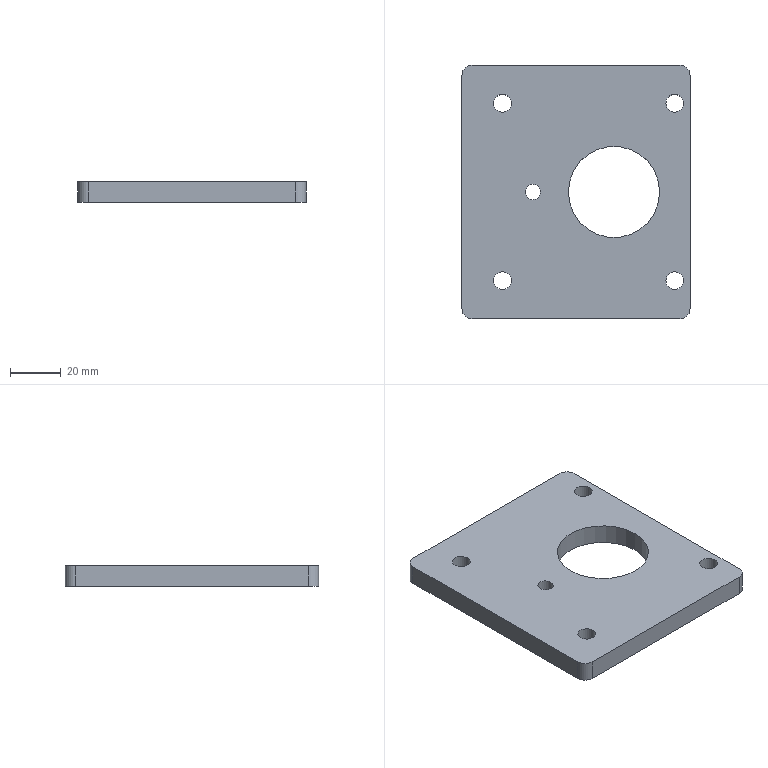Part | NX | features BREP 1, DATUM_CSYS 1 | 1 solid | 16 faces | box 90 x 100 x 8 mm | volume 62289 mm3 | cylinder 10 | plane 6 | commonest cylinder face diameters 7 x4 8 x4 6 x1 36 x1
STEP:
#1=CARTESIAN_POINT('',(0.,-46.,8.));
#2=VERTEX_POINT('',#1);
#3=CARTESIAN_POINT('',(0.,46.,8.));
#4=VERTEX_POINT('',#3);
#5=CARTESIAN_POINT('',(0.,-46.,8.));
#6=DIRECTION('',(0.,1.,0.));
#7=VECTOR('',#6,1000.);
#8=LINE('',#5,#7);
#9=EDGE_CURVE('',#2,#4,#8,.T.);
#10=ORIENTED_EDGE('',*,*,#9,.F.);
#11=CARTESIAN_POINT('',(0.,-46.,0.));
#12=VERTEX_POINT('',#11);
#13=CARTESIAN_POINT('',(0.,-46.,8.));
#14=DIRECTION('',(0.,0.,-1.));
#15=VECTOR('',#14,1000.);
#16=LINE('',#13,#15);
#17=EDGE_CURVE('',#2,#12,#16,.T.);
#18=ORIENTED_EDGE('',*,*,#17,.T.);
#19=CARTESIAN_POINT('',(0.,46.,0.));
#20=VERTEX_POINT('',#19);
#21=CARTESIAN_POINT('',(0.,-46.,0.));
#22=DIRECTION('',(0.,1.,0.));
#23=VECTOR('',#22,1000.);
#24=LINE('',#21,#23);
#25=EDGE_CURVE('',#12,#20,#24,.T.);
#26=ORIENTED_EDGE('',*,*,#25,.T.);
#27=CARTESIAN_POINT('',(0.,46.,0.));
#28=DIRECTION('',(0.,0.,1.));
#29=VECTOR('',#28,1000.);
#30=LINE('',#27,#29);
#31=EDGE_CURVE('',#20,#4,#30,.T.);
#32=ORIENTED_EDGE('',*,*,#31,.T.);
#33=EDGE_LOOP('',(#10,#18,#26,#32));
#34=FACE_BOUND('',#33,.T.);
#35=CARTESIAN_POINT('',(0.,0.,1.));
#36=DIRECTION('',(1.,0.,0.));
#37=DIRECTION('',(0.,-1.,0.));
#38=AXIS2_PLACEMENT_3D('',#35,#36,#37);
#39=PLANE('',#38);
#40=ADVANCED_FACE('',(#34),#39,.T.);
#41=CARTESIAN_POINT('',(-4.,50.,8.));
#42=VERTEX_POINT('',#41);
#43=CARTESIAN_POINT('',(-86.,50.,8.));
#44=VERTEX_POINT('',#43);
#45=CARTESIAN_POINT('',(-4.,50.,8.));
#46=DIRECTION('',(-1.,0.,0.));
#47=VECTOR('',#46,1000.);
#48=LINE('',#45,#47);
#49=EDGE_CURVE('',#42,#44,#48,.T.);
#50=ORIENTED_EDGE('',*,*,#49,.F.);
#51=CARTESIAN_POINT('',(-4.,50.,0.));
#52=VERTEX_POINT('',#51);
#53=CARTESIAN_POINT('',(-4.,50.,0.));
#54=DIRECTION('',(0.,0.,1.));
#55=VECTOR('',#54,1000.);
#56=LINE('',#53,#55);
#57=EDGE_CURVE('',#52,#42,#56,.T.);
#58=ORIENTED_EDGE('',*,*,#57,.F.);
#59=CARTESIAN_POINT('',(-86.,50.,0.));
#60=VERTEX_POINT('',#59);
#61=CARTESIAN_POINT('',(-4.,50.,0.));
#62=DIRECTION('',(-1.,0.,0.));
#63=VECTOR('',#62,1000.);
#64=LINE('',#61,#63);
#65=EDGE_CURVE('',#52,#60,#64,.T.);
#66=ORIENTED_EDGE('',*,*,#65,.T.);
#67=CARTESIAN_POINT('',(-86.,50.,0.));
#68=DIRECTION('',(0.,0.,1.));
#69=VECTOR('',#68,1000.);
#70=LINE('',#67,#69);
#71=EDGE_CURVE('',#60,#44,#70,.T.);
#72=ORIENTED_EDGE('',*,*,#71,.T.);
#73=EDGE_LOOP('',(#50,#58,#66,#72));
#74=FACE_BOUND('',#73,.T.);
#75=CARTESIAN_POINT('',(-45.,50.,1.));
#76=DIRECTION('',(0.,1.,0.));
#77=DIRECTION('',(1.,0.,0.));
#78=AXIS2_PLACEMENT_3D('',#75,#76,#77);
#79=PLANE('',#78);
#80=ADVANCED_FACE('',(#74),#79,.T.);
#81=CARTESIAN_POINT('',(-90.,-46.,8.));
#82=VERTEX_POINT('',#81);
#83=CARTESIAN_POINT('',(-90.,46.,8.));
#84=VERTEX_POINT('',#83);
#85=CARTESIAN_POINT('',(-90.,-46.,8.));
#86=DIRECTION('',(0.,1.,0.));
#87=VECTOR('',#86,1000.);
#88=LINE('',#85,#87);
#89=EDGE_CURVE('',#82,#84,#88,.T.);
#90=ORIENTED_EDGE('',*,*,#89,.T.);
#91=CARTESIAN_POINT('',(-90.,46.,0.));
#92=VERTEX_POINT('',#91);
#93=CARTESIAN_POINT('',(-90.,46.,0.));
#94=DIRECTION('',(0.,0.,1.));
#95=VECTOR('',#94,1000.);
#96=LINE('',#93,#95);
#97=EDGE_CURVE('',#92,#84,#96,.T.);
#98=ORIENTED_EDGE('',*,*,#97,.F.);
#99=CARTESIAN_POINT('',(-90.,-46.,0.));
#100=VERTEX_POINT('',#99);
#101=CARTESIAN_POINT('',(-90.,-46.,0.));
#102=DIRECTION('',(0.,1.,0.));
#103=VECTOR('',#102,1000.);
#104=LINE('',#101,#103);
#105=EDGE_CURVE('',#100,#92,#104,.T.);
#106=ORIENTED_EDGE('',*,*,#105,.F.);
#107=CARTESIAN_POINT('',(-90.,-46.,0.));
#108=DIRECTION('',(0.,0.,1.));
#109=VECTOR('',#108,1000.);
#110=LINE('',#107,#109);
#111=EDGE_CURVE('',#100,#82,#110,.T.);
#112=ORIENTED_EDGE('',*,*,#111,.T.);
#113=EDGE_LOOP('',(#90,#98,#106,#112));
#114=FACE_BOUND('',#113,.T.);
#115=CARTESIAN_POINT('',(-90.,0.,1.));
#116=DIRECTION('',(-1.,0.,0.));
#117=DIRECTION('',(0.,1.,0.));
#118=AXIS2_PLACEMENT_3D('',#115,#116,#117);
#119=PLANE('',#118);
#120=ADVANCED_FACE('',(#114),#119,.T.);
#121=CARTESIAN_POINT('',(-86.,-50.,0.));
#122=VERTEX_POINT('',#121);
#123=CARTESIAN_POINT('',(-4.,-50.,0.));
#124=VERTEX_POINT('',#123);
#125=CARTESIAN_POINT('',(-86.,-50.,0.));
#126=DIRECTION('',(1.,0.,0.));
#127=VECTOR('',#126,1000.);
#128=LINE('',#125,#127);
#129=EDGE_CURVE('',#122,#124,#128,.T.);
#130=ORIENTED_EDGE('',*,*,#129,.T.);
#131=CARTESIAN_POINT('',(-4.,-50.,8.));
#132=VERTEX_POINT('',#131);
#133=CARTESIAN_POINT('',(-4.,-50.,8.));
#134=DIRECTION('',(0.,0.,-1.));
#135=VECTOR('',#134,1000.);
#136=LINE('',#133,#135);
#137=EDGE_CURVE('',#132,#124,#136,.T.);
#138=ORIENTED_EDGE('',*,*,#137,.F.);
#139=CARTESIAN_POINT('',(-86.,-50.,8.));
#140=VERTEX_POINT('',#139);
#141=CARTESIAN_POINT('',(-86.,-50.,8.));
#142=DIRECTION('',(1.,0.,0.));
#143=VECTOR('',#142,1000.);
#144=LINE('',#141,#143);
#145=EDGE_CURVE('',#140,#132,#144,.T.);
#146=ORIENTED_EDGE('',*,*,#145,.F.);
#147=CARTESIAN_POINT('',(-86.,-50.,0.));
#148=DIRECTION('',(0.,0.,1.));
#149=VECTOR('',#148,1000.);
#150=LINE('',#147,#149);
#151=EDGE_CURVE('',#122,#140,#150,.T.);
#152=ORIENTED_EDGE('',*,*,#151,.F.);
#153=EDGE_LOOP('',(#130,#138,#146,#152));
#154=FACE_BOUND('',#153,.T.);
#155=CARTESIAN_POINT('',(-45.,-50.,1.));
#156=DIRECTION('',(0.,-1.,0.));
#157=DIRECTION('',(-1.,0.,0.));
#158=AXIS2_PLACEMENT_3D('',#155,#156,#157);
#159=PLANE('',#158);
#160=ADVANCED_FACE('',(#154),#159,.T.);
#161=CARTESIAN_POINT('',(-2.5,-35.,0.));
#162=VERTEX_POINT('',#161);
#163=CARTESIAN_POINT('',(-2.5,-35.,8.));
#164=VERTEX_POINT('',#163);
#165=CARTESIAN_POINT('',(-2.5,-35.,0.));
#166=DIRECTION('',(0.,0.,1.));
#167=VECTOR('',#166,1000.);
#168=LINE('',#165,#167);
#169=EDGE_CURVE('',#162,#164,#168,.T.);
#170=ORIENTED_EDGE('',*,*,#169,.T.);
#171=CARTESIAN_POINT('',(-6.,-35.,8.));
#172=DIRECTION('',(0.,0.,1.));
#173=DIRECTION('',(1.,0.,0.));
#174=AXIS2_PLACEMENT_3D('',#171,#172,#173);
#175=CIRCLE('',#174,3.5);
#176=EDGE_CURVE('',#164,#164,#175,.T.);
#177=ORIENTED_EDGE('',*,*,#176,.T.);
#178=ORIENTED_EDGE('',*,*,#169,.F.);
#179=CARTESIAN_POINT('',(-6.,-35.,0.));
#180=DIRECTION('',(0.,0.,1.));
#181=DIRECTION('',(1.,0.,0.));
#182=AXIS2_PLACEMENT_3D('',#179,#180,#181);
#183=CIRCLE('',#182,3.5);
#184=EDGE_CURVE('',#162,#162,#183,.T.);
#185=ORIENTED_EDGE('',*,*,#184,.F.);
#186=EDGE_LOOP('',(#170,#177,#178,#185));
#187=FACE_BOUND('',#186,.T.);
#188=CARTESIAN_POINT('',(-6.,-35.,0.));
#189=DIRECTION('',(0.,0.,1.));
#190=DIRECTION('',(-1.,0.,0.));
#191=AXIS2_PLACEMENT_3D('',#188,#189,#190);
#192=CYLINDRICAL_SURFACE('',#191,3.5);
#193=ADVANCED_FACE('',(#187),#192,.F.);
#194=CARTESIAN_POINT('',(-2.5,35.,0.));
#195=VERTEX_POINT('',#194);
#196=CARTESIAN_POINT('',(-2.5,35.,8.));
#197=VERTEX_POINT('',#196);
#198=CARTESIAN_POINT('',(-2.5,35.,0.));
#199=DIRECTION('',(0.,0.,1.));
#200=VECTOR('',#199,1000.);
#201=LINE('',#198,#200);
#202=EDGE_CURVE('',#195,#197,#201,.T.);
#203=ORIENTED_EDGE('',*,*,#202,.T.);
#204=CARTESIAN_POINT('',(-6.,35.,8.));
#205=DIRECTION('',(0.,0.,1.));
#206=DIRECTION('',(1.,0.,0.));
#207=AXIS2_PLACEMENT_3D('',#204,#205,#206);
#208=CIRCLE('',#207,3.5);
#209=EDGE_CURVE('',#197,#197,#208,.T.);
#210=ORIENTED_EDGE('',*,*,#209,.T.);
#211=ORIENTED_EDGE('',*,*,#202,.F.);
#212=CARTESIAN_POINT('',(-6.,35.,0.));
#213=DIRECTION('',(0.,0.,1.));
#214=DIRECTION('',(1.,0.,0.));
#215=AXIS2_PLACEMENT_3D('',#212,#213,#214);
#216=CIRCLE('',#215,3.5);
#217=EDGE_CURVE('',#195,#195,#216,.T.);
#218=ORIENTED_EDGE('',*,*,#217,.F.);
#219=EDGE_LOOP('',(#203,#210,#211,#218));
#220=FACE_BOUND('',#219,.T.);
#221=CARTESIAN_POINT('',(-6.,35.,0.));
#222=DIRECTION('',(0.,0.,1.));
#223=DIRECTION('',(-1.,0.,0.));
#224=AXIS2_PLACEMENT_3D('',#221,#222,#223);
#225=CYLINDRICAL_SURFACE('',#224,3.5);
#226=ADVANCED_FACE('',(#220),#225,.F.);
#227=CARTESIAN_POINT('',(-70.5,35.,0.));
#228=VERTEX_POINT('',#227);
#229=CARTESIAN_POINT('',(-70.5,35.,8.));
#230=VERTEX_POINT('',#229);
#231=CARTESIAN_POINT('',(-70.5,35.,0.));
#232=DIRECTION('',(0.,0.,1.));
#233=VECTOR('',#232,1000.);
#234=LINE('',#231,#233);
#235=EDGE_CURVE('',#228,#230,#234,.T.);
#236=ORIENTED_EDGE('',*,*,#235,.T.);
#237=CARTESIAN_POINT('',(-74.,35.,8.));
#238=DIRECTION('',(0.,0.,1.));
#239=DIRECTION('',(1.,0.,0.));
#240=AXIS2_PLACEMENT_3D('',#237,#238,#239);
#241=CIRCLE('',#240,3.5);
#242=EDGE_CURVE('',#230,#230,#241,.T.);
#243=ORIENTED_EDGE('',*,*,#242,.T.);
#244=ORIENTED_EDGE('',*,*,#235,.F.);
#245=CARTESIAN_POINT('',(-74.,35.,0.));
#246=DIRECTION('',(0.,0.,1.));
#247=DIRECTION('',(1.,0.,0.));
#248=AXIS2_PLACEMENT_3D('',#245,#246,#247);
#249=CIRCLE('',#248,3.5);
#250=EDGE_CURVE('',#228,#228,#249,.T.);
#251=ORIENTED_EDGE('',*,*,#250,.F.);
#252=EDGE_LOOP('',(#236,#243,#244,#251));
#253=FACE_BOUND('',#252,.T.);
#254=CARTESIAN_POINT('',(-74.,35.,0.));
#255=DIRECTION('',(0.,0.,1.));
#256=DIRECTION('',(-1.,0.,0.));
#257=AXIS2_PLACEMENT_3D('',#254,#255,#256);
#258=CYLINDRICAL_SURFACE('',#257,3.5);
#259=ADVANCED_FACE('',(#253),#258,.F.);
#260=CARTESIAN_POINT('',(-70.5,-35.,0.));
#261=VERTEX_POINT('',#260);
#262=CARTESIAN_POINT('',(-70.5,-35.,8.));
#263=VERTEX_POINT('',#262);
#264=CARTESIAN_POINT('',(-70.5,-35.,0.));
#265=DIRECTION('',(0.,0.,1.));
#266=VECTOR('',#265,1000.);
#267=LINE('',#264,#266);
#268=EDGE_CURVE('',#261,#263,#267,.T.);
#269=ORIENTED_EDGE('',*,*,#268,.T.);
#270=CARTESIAN_POINT('',(-74.,-35.,8.));
#271=DIRECTION('',(0.,0.,1.));
#272=DIRECTION('',(1.,0.,0.));
#273=AXIS2_PLACEMENT_3D('',#270,#271,#272);
#274=CIRCLE('',#273,3.5);
#275=EDGE_CURVE('',#263,#263,#274,.T.);
#276=ORIENTED_EDGE('',*,*,#275,.T.);
#277=ORIENTED_EDGE('',*,*,#268,.F.);
#278=CARTESIAN_POINT('',(-74.,-35.,0.));
#279=DIRECTION('',(0.,0.,1.));
#280=DIRECTION('',(1.,0.,0.));
#281=AXIS2_PLACEMENT_3D('',#278,#279,#280);
#282=CIRCLE('',#281,3.5);
#283=EDGE_CURVE('',#261,#261,#282,.T.);
#284=ORIENTED_EDGE('',*,*,#283,.F.);
#285=EDGE_LOOP('',(#269,#276,#277,#284));
#286=FACE_BOUND('',#285,.T.);
#287=CARTESIAN_POINT('',(-74.,-35.,0.));
#288=DIRECTION('',(0.,0.,1.));
#289=DIRECTION('',(-1.,0.,0.));
#290=AXIS2_PLACEMENT_3D('',#287,#288,#289);
#291=CYLINDRICAL_SURFACE('',#290,3.5);
#292=ADVANCED_FACE('',(#286),#291,.F.);
#293=CARTESIAN_POINT('',(-86.,-46.,0.));
#294=DIRECTION('',(0.,0.,1.));
#295=DIRECTION('',(-1.,0.,0.));
#296=AXIS2_PLACEMENT_3D('',#293,#294,#295);
#297=CIRCLE('',#296,4.);
#298=EDGE_CURVE('',#100,#122,#297,.T.);
#299=ORIENTED_EDGE('',*,*,#298,.F.);
#300=ORIENTED_EDGE('',*,*,#105,.T.);
#301=CARTESIAN_POINT('',(-86.,46.,0.));
#302=DIRECTION('',(0.,0.,-1.));
#303=DIRECTION('',(-1.,0.,0.));
#304=AXIS2_PLACEMENT_3D('',#301,#302,#303);
#305=CIRCLE('',#304,4.);
#306=EDGE_CURVE('',#92,#60,#305,.T.);
#307=ORIENTED_EDGE('',*,*,#306,.T.);
#308=ORIENTED_EDGE('',*,*,#65,.F.);
#309=CARTESIAN_POINT('',(-4.,46.,0.));
#310=DIRECTION('',(0.,0.,-1.));
#311=DIRECTION('',(0.,1.,0.));
#312=AXIS2_PLACEMENT_3D('',#309,#310,#311);
#313=CIRCLE('',#312,4.);
#314=EDGE_CURVE('',#52,#20,#313,.T.);
#315=ORIENTED_EDGE('',*,*,#314,.T.);
#316=ORIENTED_EDGE('',*,*,#25,.F.);
#317=CARTESIAN_POINT('',(-4.,-46.,0.));
#318=DIRECTION('',(0.,0.,-1.));
#319=DIRECTION('',(1.,0.,0.));
#320=AXIS2_PLACEMENT_3D('',#317,#318,#319);
#321=CIRCLE('',#320,4.);
#322=EDGE_CURVE('',#12,#124,#321,.T.);
#323=ORIENTED_EDGE('',*,*,#322,.T.);
#324=ORIENTED_EDGE('',*,*,#129,.F.);
#325=EDGE_LOOP('',(#299,#300,#307,#308,#315,#316,#323,#324));
#326=FACE_BOUND('',#325,.T.);
#327=CARTESIAN_POINT('',(-12.,0.,0.));
#328=VERTEX_POINT('',#327);
#329=CARTESIAN_POINT('',(-30.,0.,0.));
#330=DIRECTION('',(0.,0.,-1.));
#331=DIRECTION('',(1.,0.,0.));
#332=AXIS2_PLACEMENT_3D('',#329,#330,#331);
#333=CIRCLE('',#332,18.);
#334=EDGE_CURVE('',#328,#328,#333,.T.);
#335=ORIENTED_EDGE('',*,*,#334,.F.);
#336=EDGE_LOOP('',(#335));
#337=FACE_BOUND('',#336,.T.);
#338=CARTESIAN_POINT('',(-59.,0.,0.));
#339=VERTEX_POINT('',#338);
#340=CARTESIAN_POINT('',(-62.,0.,0.));
#341=DIRECTION('',(0.,0.,-1.));
#342=DIRECTION('',(1.,0.,0.));
#343=AXIS2_PLACEMENT_3D('',#340,#341,#342);
#344=CIRCLE('',#343,3.);
#345=EDGE_CURVE('',#339,#339,#344,.T.);
#346=ORIENTED_EDGE('',*,*,#345,.F.);
#347=EDGE_LOOP('',(#346));
#348=FACE_BOUND('',#347,.T.);
#349=ORIENTED_EDGE('',*,*,#184,.T.);
#350=EDGE_LOOP('',(#349));
#351=FACE_BOUND('',#350,.T.);
#352=ORIENTED_EDGE('',*,*,#217,.T.);
#353=EDGE_LOOP('',(#352));
#354=FACE_BOUND('',#353,.T.);
#355=ORIENTED_EDGE('',*,*,#250,.T.);
#356=EDGE_LOOP('',(#355));
#357=FACE_BOUND('',#356,.T.);
#358=ORIENTED_EDGE('',*,*,#283,.T.);
#359=EDGE_LOOP('',(#358));
#360=FACE_BOUND('',#359,.T.);
#361=CARTESIAN_POINT('',(-45.,0.1084,0.));
#362=DIRECTION('',(0.,0.,1.));
#363=DIRECTION('',(-1.,0.,0.));
#364=AXIS2_PLACEMENT_3D('',#361,#362,#363);
#365=PLANE('',#364);
#366=ADVANCED_FACE('',(#326,#337,#348,#351,#354,#357,#360),#365,.F.);
#367=ORIENTED_EDGE('',*,*,#145,.T.);
#368=CARTESIAN_POINT('',(-4.,-46.,8.));
#369=DIRECTION('',(0.,0.,-1.));
#370=DIRECTION('',(1.,0.,0.));
#371=AXIS2_PLACEMENT_3D('',#368,#369,#370);
#372=CIRCLE('',#371,4.);
#373=EDGE_CURVE('',#2,#132,#372,.T.);
#374=ORIENTED_EDGE('',*,*,#373,.F.);
#375=ORIENTED_EDGE('',*,*,#9,.T.);
#376=CARTESIAN_POINT('',(-4.,46.,8.));
#377=DIRECTION('',(0.,0.,-1.));
#378=DIRECTION('',(0.,1.,0.));
#379=AXIS2_PLACEMENT_3D('',#376,#377,#378);
#380=CIRCLE('',#379,4.);
#381=EDGE_CURVE('',#42,#4,#380,.T.);
#382=ORIENTED_EDGE('',*,*,#381,.F.);
#383=ORIENTED_EDGE('',*,*,#49,.T.);
#384=CARTESIAN_POINT('',(-86.,46.,8.));
#385=DIRECTION('',(0.,0.,-1.));
#386=DIRECTION('',(-1.,0.,0.));
#387=AXIS2_PLACEMENT_3D('',#384,#385,#386);
#388=CIRCLE('',#387,4.);
#389=EDGE_CURVE('',#84,#44,#388,.T.);
#390=ORIENTED_EDGE('',*,*,#389,.F.);
#391=ORIENTED_EDGE('',*,*,#89,.F.);
#392=CARTESIAN_POINT('',(-86.,-46.,8.));
#393=DIRECTION('',(0.,0.,1.));
#394=DIRECTION('',(-1.,0.,0.));
#395=AXIS2_PLACEMENT_3D('',#392,#393,#394);
#396=CIRCLE('',#395,4.);
#397=EDGE_CURVE('',#82,#140,#396,.T.);
#398=ORIENTED_EDGE('',*,*,#397,.T.);
#399=EDGE_LOOP('',(#367,#374,#375,#382,#383,#390,#391,#398));
#400=FACE_BOUND('',#399,.T.);
#401=CARTESIAN_POINT('',(-12.,0.,8.));
#402=VERTEX_POINT('',#401);
#403=CARTESIAN_POINT('',(-30.,0.,8.));
#404=DIRECTION('',(0.,0.,1.));
#405=DIRECTION('',(1.,0.,0.));
#406=AXIS2_PLACEMENT_3D('',#403,#404,#405);
#407=CIRCLE('',#406,18.);
#408=EDGE_CURVE('',#402,#402,#407,.T.);
#409=ORIENTED_EDGE('',*,*,#408,.F.);
#410=EDGE_LOOP('',(#409));
#411=FACE_BOUND('',#410,.T.);
#412=CARTESIAN_POINT('',(-59.,0.,8.));
#413=VERTEX_POINT('',#412);
#414=CARTESIAN_POINT('',(-62.,0.,8.));
#415=DIRECTION('',(0.,0.,1.));
#416=DIRECTION('',(1.,0.,0.));
#417=AXIS2_PLACEMENT_3D('',#414,#415,#416);
#418=CIRCLE('',#417,3.);
#419=EDGE_CURVE('',#413,#413,#418,.T.);
#420=ORIENTED_EDGE('',*,*,#419,.F.);
#421=EDGE_LOOP('',(#420));
#422=FACE_BOUND('',#421,.T.);
#423=ORIENTED_EDGE('',*,*,#176,.F.);
#424=EDGE_LOOP('',(#423));
#425=FACE_BOUND('',#424,.T.);
#426=ORIENTED_EDGE('',*,*,#209,.F.);
#427=EDGE_LOOP('',(#426));
#428=FACE_BOUND('',#427,.T.);
#429=ORIENTED_EDGE('',*,*,#242,.F.);
#430=EDGE_LOOP('',(#429));
#431=FACE_BOUND('',#430,.T.);
#432=ORIENTED_EDGE('',*,*,#275,.F.);
#433=EDGE_LOOP('',(#432));
#434=FACE_BOUND('',#433,.T.);
#435=CARTESIAN_POINT('',(-45.,0.1084,8.));
#436=DIRECTION('',(0.,0.,1.));
#437=DIRECTION('',(-1.,0.,0.));
#438=AXIS2_PLACEMENT_3D('',#435,#436,#437);
#439=PLANE('',#438);
#440=ADVANCED_FACE('',(#400,#411,#422,#425,#428,#431,#434),#439,.T.);
#441=ORIENTED_EDGE('',*,*,#419,.T.);
#442=CARTESIAN_POINT('',(-59.,0.,8.));
#443=DIRECTION('',(0.,0.,-1.));
#444=VECTOR('',#443,1000.);
#445=LINE('',#442,#444);
#446=EDGE_CURVE('',#413,#339,#445,.T.);
#447=ORIENTED_EDGE('',*,*,#446,.T.);
#448=ORIENTED_EDGE('',*,*,#345,.T.);
#449=ORIENTED_EDGE('',*,*,#446,.F.);
#450=EDGE_LOOP('',(#441,#447,#448,#449));
#451=FACE_BOUND('',#450,.T.);
#452=CARTESIAN_POINT('',(-62.,0.,8.));
#453=DIRECTION('',(0.,0.,-1.));
#454=DIRECTION('',(-1.,0.,0.));
#455=AXIS2_PLACEMENT_3D('',#452,#453,#454);
#456=CYLINDRICAL_SURFACE('',#455,3.);
#457=ADVANCED_FACE('',(#451),#456,.F.);
#458=ORIENTED_EDGE('',*,*,#408,.T.);
#459=CARTESIAN_POINT('',(-12.,0.,8.));
#460=DIRECTION('',(0.,0.,-1.));
#461=VECTOR('',#460,1000.);
#462=LINE('',#459,#461);
#463=EDGE_CURVE('',#402,#328,#462,.T.);
#464=ORIENTED_EDGE('',*,*,#463,.T.);
#465=ORIENTED_EDGE('',*,*,#334,.T.);
#466=ORIENTED_EDGE('',*,*,#463,.F.);
#467=EDGE_LOOP('',(#458,#464,#465,#466));
#468=FACE_BOUND('',#467,.T.);
#469=CARTESIAN_POINT('',(-30.,0.,8.));
#470=DIRECTION('',(0.,0.,-1.));
#471=DIRECTION('',(-1.,0.,0.));
#472=AXIS2_PLACEMENT_3D('',#469,#470,#471);
#473=CYLINDRICAL_SURFACE('',#472,18.);
#474=ADVANCED_FACE('',(#468),#473,.F.);
#475=ORIENTED_EDGE('',*,*,#373,.T.);
#476=ORIENTED_EDGE('',*,*,#137,.T.);
#477=ORIENTED_EDGE('',*,*,#322,.F.);
#478=ORIENTED_EDGE('',*,*,#17,.F.);
#479=EDGE_LOOP('',(#475,#476,#477,#478));
#480=FACE_BOUND('',#479,.T.);
#481=CARTESIAN_POINT('',(-4.,-46.,8.));
#482=DIRECTION('',(0.,0.,-1.));
#483=DIRECTION('',(-1.,0.,0.));
#484=AXIS2_PLACEMENT_3D('',#481,#482,#483);
#485=CYLINDRICAL_SURFACE('',#484,4.);
#486=ADVANCED_FACE('',(#480),#485,.T.);
#487=ORIENTED_EDGE('',*,*,#31,.F.);
#488=ORIENTED_EDGE('',*,*,#314,.F.);
#489=ORIENTED_EDGE('',*,*,#57,.T.);
#490=ORIENTED_EDGE('',*,*,#381,.T.);
#491=EDGE_LOOP('',(#487,#488,#489,#490));
#492=FACE_BOUND('',#491,.T.);
#493=CARTESIAN_POINT('',(-4.,46.,-2.777));
#494=DIRECTION('',(0.,0.,1.));
#495=DIRECTION('',(0.,-1.,0.));
#496=AXIS2_PLACEMENT_3D('',#493,#494,#495);
#497=CYLINDRICAL_SURFACE('',#496,4.);
#498=ADVANCED_FACE('',(#492),#497,.T.);
#499=ORIENTED_EDGE('',*,*,#71,.F.);
#500=ORIENTED_EDGE('',*,*,#306,.F.);
#501=ORIENTED_EDGE('',*,*,#97,.T.);
#502=ORIENTED_EDGE('',*,*,#389,.T.);
#503=EDGE_LOOP('',(#499,#500,#501,#502));
#504=FACE_BOUND('',#503,.T.);
#505=CARTESIAN_POINT('',(-86.,46.,-2.777));
#506=DIRECTION('',(0.,0.,1.));
#507=DIRECTION('',(1.,0.,0.));
#508=AXIS2_PLACEMENT_3D('',#505,#506,#507);
#509=CYLINDRICAL_SURFACE('',#508,4.);
#510=ADVANCED_FACE('',(#504),#509,.T.);
#511=ORIENTED_EDGE('',*,*,#397,.F.);
#512=ORIENTED_EDGE('',*,*,#111,.F.);
#513=ORIENTED_EDGE('',*,*,#298,.T.);
#514=ORIENTED_EDGE('',*,*,#151,.T.);
#515=EDGE_LOOP('',(#511,#512,#513,#514));
#516=FACE_BOUND('',#515,.T.);
#517=CARTESIAN_POINT('',(-86.,-46.,-2.777));
#518=DIRECTION('',(0.,0.,1.));
#519=DIRECTION('',(1.,0.,0.));
#520=AXIS2_PLACEMENT_3D('',#517,#518,#519);
#521=CYLINDRICAL_SURFACE('',#520,4.);
#522=ADVANCED_FACE('',(#516),#521,.T.);
#523=CLOSED_SHELL('',(#40,#80,#120,#160,#193,#226,#259,#292,#366,#440,#457,#474,#486,#498,#510,#522));
#524=MANIFOLD_SOLID_BREP('',#523);
#525=(LENGTH_UNIT()NAMED_UNIT(*)SI_UNIT(.MILLI.,.METRE.));
#526=UNCERTAINTY_MEASURE_WITH_UNIT(LENGTH_MEASURE(0.00001),#525,'','');
#527=(NAMED_UNIT(*)PLANE_ANGLE_UNIT()SI_UNIT($,.RADIAN.));
#528=(NAMED_UNIT(*)SI_UNIT($,.STERADIAN.)SOLID_ANGLE_UNIT());
#529=(GEOMETRIC_REPRESENTATION_CONTEXT(3)GLOBAL_UNCERTAINTY_ASSIGNED_CONTEXT((#526))GLOBAL_UNIT_ASSIGNED_CONTEXT((#525,#527,#528))REPRESENTATION_CONTEXT('',''));
#530=ADVANCED_BREP_SHAPE_REPRESENTATION('',(#524),#529);